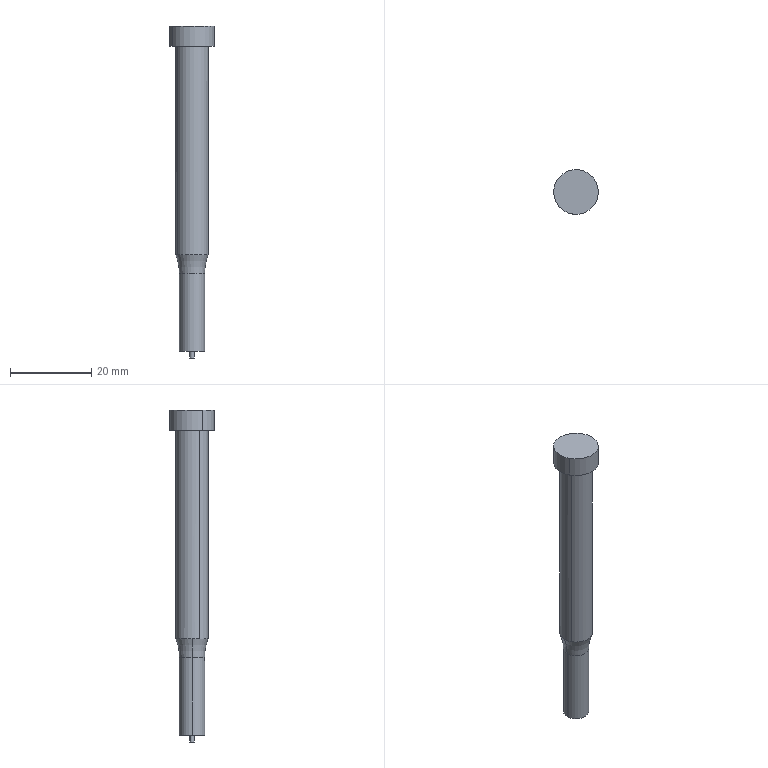Part | CATIA | 1 solid | 14 faces | box 11 x 11 x 81.7 mm | volume 3799 mm3 | cylinder 8 | plane 4 | torus 2 | commonest cylinder face diameters 1.04 x2 6.2 x2 8 x2 11 x2
STEP:
#1=CARTESIAN_POINT('',(3.1,0.,0.));
#2=VERTEX_POINT('',#1);
#3=CARTESIAN_POINT('',(-3.1,0.,0.));
#4=VERTEX_POINT('',#3);
#5=CARTESIAN_POINT('',(0.,0.,0.));
#6=DIRECTION('',(0.,0.,1.));
#7=AXIS2_PLACEMENT_3D('',#5,#6,$);
#8=CIRCLE('',#7,3.1);
#9=EDGE_CURVE('',#2,#4,#8,.T.);
#10=ORIENTED_EDGE('',*,*,#9,.F.);
#11=CARTESIAN_POINT('',(0.,0.,0.));
#12=DIRECTION('',(0.,0.,1.));
#13=AXIS2_PLACEMENT_3D('',#11,#12,$);
#14=CIRCLE('',#13,3.1);
#15=EDGE_CURVE('',#4,#2,#14,.T.);
#16=ORIENTED_EDGE('',*,*,#15,.F.);
#17=EDGE_LOOP('',(#10,#16));
#18=FACE_OUTER_BOUND('',#17,.T.);
#19=CARTESIAN_POINT('',(0.4563,-0.2493,0.));
#20=VERTEX_POINT('',#19);
#21=CARTESIAN_POINT('',(-0.4563,0.2493,0.));
#22=VERTEX_POINT('',#21);
#23=CARTESIAN_POINT('',(0.,0.,0.));
#24=DIRECTION('',(0.,0.,1.));
#25=AXIS2_PLACEMENT_3D('',#23,#24,$);
#26=CIRCLE('',#25,0.52);
#27=EDGE_CURVE('',#20,#22,#26,.F.);
#28=ORIENTED_EDGE('',*,*,#27,.F.);
#29=CARTESIAN_POINT('',(0.,0.,0.));
#30=DIRECTION('',(0.,0.,1.));
#31=AXIS2_PLACEMENT_3D('',#29,#30,$);
#32=CIRCLE('',#31,0.52);
#33=EDGE_CURVE('',#22,#20,#32,.F.);
#34=ORIENTED_EDGE('',*,*,#33,.F.);
#35=EDGE_LOOP('',(#28,#34));
#36=FACE_BOUND('',#35,.T.);
#37=CARTESIAN_POINT('',(4.,0.,0.));
#38=DIRECTION('',(0.,0.,1.));
#39=DIRECTION('',(1.,0.,0.));
#40=AXIS2_PLACEMENT_3D('',#37,#38,#39);
#41=PLANE('',#40);
#42=ADVANCED_FACE('',(#18,#36),#41,.F.);
#43=CARTESIAN_POINT('',(-4.,0.,23.753));
#44=VERTEX_POINT('',#43);
#45=CARTESIAN_POINT('',(3.51,1.918,23.753));
#46=VERTEX_POINT('',#45);
#47=CARTESIAN_POINT('',(0.,0.,23.753));
#48=DIRECTION('',(0.,0.,-1.));
#49=AXIS2_PLACEMENT_3D('',#47,#48,$);
#50=CIRCLE('',#49,4.);
#51=EDGE_CURVE('',#44,#46,#50,.T.);
#52=ORIENTED_EDGE('',*,*,#51,.T.);
#53=CARTESIAN_POINT('',(4.,0.,23.753));
#54=VERTEX_POINT('',#53);
#55=CARTESIAN_POINT('',(0.,0.,23.753));
#56=DIRECTION('',(0.,0.,-1.));
#57=AXIS2_PLACEMENT_3D('',#55,#56,$);
#58=CIRCLE('',#57,4.);
#59=EDGE_CURVE('',#54,#46,#58,.F.);
#60=ORIENTED_EDGE('',*,*,#59,.F.);
#61=CARTESIAN_POINT('',(3.1,0.,19.));
#62=VERTEX_POINT('',#61);
#63=CARTESIAN_POINT('',(16.1,0.,19.));
#64=DIRECTION('',(0.,1.,0.));
#65=AXIS2_PLACEMENT_3D('',#63,#64,$);
#66=CIRCLE('',#65,13.);
#67=EDGE_CURVE('',#54,#62,#66,.F.);
#68=ORIENTED_EDGE('',*,*,#67,.T.);
#69=CARTESIAN_POINT('',(-3.1,0.,19.));
#70=VERTEX_POINT('',#69);
#71=CARTESIAN_POINT('',(0.,0.,19.));
#72=DIRECTION('',(0.,0.,-1.));
#73=AXIS2_PLACEMENT_3D('',#71,#72,$);
#74=CIRCLE('',#73,3.1);
#75=EDGE_CURVE('',#70,#62,#74,.T.);
#76=ORIENTED_EDGE('',*,*,#75,.F.);
#77=CARTESIAN_POINT('',(-16.1,0.,19.));
#78=DIRECTION('',(0.,-1.,0.));
#79=AXIS2_PLACEMENT_3D('',#77,#78,$);
#80=CIRCLE('',#79,13.);
#81=EDGE_CURVE('',#44,#70,#80,.F.);
#82=ORIENTED_EDGE('',*,*,#81,.F.);
#83=EDGE_LOOP('',(#52,#60,#68,#76,#82));
#84=FACE_OUTER_BOUND('',#83,.T.);
#85=CARTESIAN_POINT('',(0.,0.,19.));
#86=DIRECTION('',(0.,0.,-1.));
#87=DIRECTION('',(-0.9862,-0.1654,0.));
#88=AXIS2_PLACEMENT_3D('',#85,#86,#87);
#89=TOROIDAL_SURFACE('',#88,16.1,13.);
#90=ADVANCED_FACE('',(#84),#89,.F.);
#91=CARTESIAN_POINT('',(-3.51,-1.918,23.753));
#92=VERTEX_POINT('',#91);
#93=CARTESIAN_POINT('',(0.,0.,23.753));
#94=DIRECTION('',(0.,0.,-1.));
#95=AXIS2_PLACEMENT_3D('',#93,#94,$);
#96=CIRCLE('',#95,4.);
#97=EDGE_CURVE('',#54,#92,#96,.T.);
#98=ORIENTED_EDGE('',*,*,#97,.T.);
#99=CARTESIAN_POINT('',(0.,0.,23.753));
#100=DIRECTION('',(0.,0.,-1.));
#101=AXIS2_PLACEMENT_3D('',#99,#100,$);
#102=CIRCLE('',#101,4.);
#103=EDGE_CURVE('',#44,#92,#102,.F.);
#104=ORIENTED_EDGE('',*,*,#103,.F.);
#105=ORIENTED_EDGE('',*,*,#81,.T.);
#106=CARTESIAN_POINT('',(0.,0.,19.));
#107=DIRECTION('',(0.,0.,-1.));
#108=AXIS2_PLACEMENT_3D('',#106,#107,$);
#109=CIRCLE('',#108,3.1);
#110=EDGE_CURVE('',#62,#70,#109,.T.);
#111=ORIENTED_EDGE('',*,*,#110,.F.);
#112=ORIENTED_EDGE('',*,*,#67,.F.);
#113=EDGE_LOOP('',(#98,#104,#105,#111,#112));
#114=FACE_OUTER_BOUND('',#113,.T.);
#115=CARTESIAN_POINT('',(0.,0.,19.));
#116=DIRECTION('',(0.,0.,-1.));
#117=DIRECTION('',(0.9734,0.2293,0.));
#118=AXIS2_PLACEMENT_3D('',#115,#116,#117);
#119=TOROIDAL_SURFACE('',#118,16.1,13.);
#120=ADVANCED_FACE('',(#114),#119,.F.);
#121=CARTESIAN_POINT('',(3.1,0.,16.61));
#122=DIRECTION('',(0.,0.,1.));
#123=VECTOR('',#122,1.);
#124=LINE('',#121,#123);
#125=EDGE_CURVE('',#2,#62,#124,.T.);
#126=ORIENTED_EDGE('',*,*,#125,.F.);
#127=ORIENTED_EDGE('',*,*,#9,.T.);
#128=CARTESIAN_POINT('',(-3.1,0.,16.61));
#129=DIRECTION('',(0.,0.,1.));
#130=VECTOR('',#129,1.);
#131=LINE('',#128,#130);
#132=EDGE_CURVE('',#4,#70,#131,.T.);
#133=ORIENTED_EDGE('',*,*,#132,.T.);
#134=ORIENTED_EDGE('',*,*,#75,.T.);
#135=EDGE_LOOP('',(#126,#127,#133,#134));
#136=FACE_OUTER_BOUND('',#135,.T.);
#137=CARTESIAN_POINT('',(0.,0.,16.61));
#138=DIRECTION('',(0.,0.,1.));
#139=DIRECTION('',(1.,0.,0.));
#140=AXIS2_PLACEMENT_3D('',#137,#138,#139);
#141=CYLINDRICAL_SURFACE('',#140,3.1);
#142=ADVANCED_FACE('',(#136),#141,.T.);
#143=ORIENTED_EDGE('',*,*,#132,.F.);
#144=ORIENTED_EDGE('',*,*,#15,.T.);
#145=ORIENTED_EDGE('',*,*,#125,.T.);
#146=ORIENTED_EDGE('',*,*,#110,.T.);
#147=EDGE_LOOP('',(#143,#144,#145,#146));
#148=FACE_OUTER_BOUND('',#147,.T.);
#149=CARTESIAN_POINT('',(0.,0.,16.61));
#150=DIRECTION('',(0.,0.,1.));
#151=DIRECTION('',(-1.,0.,0.));
#152=AXIS2_PLACEMENT_3D('',#149,#150,#151);
#153=CYLINDRICAL_SURFACE('',#152,3.1);
#154=ADVANCED_FACE('',(#148),#153,.T.);
#155=CARTESIAN_POINT('',(-3.51,-1.918,75.));
#156=VERTEX_POINT('',#155);
#157=CARTESIAN_POINT('',(-3.51,-1.918,37.5));
#158=DIRECTION('',(0.,0.,1.));
#159=VECTOR('',#158,1.);
#160=LINE('',#157,#159);
#161=EDGE_CURVE('',#92,#156,#160,.T.);
#162=ORIENTED_EDGE('',*,*,#161,.T.);
#163=CARTESIAN_POINT('',(3.51,1.918,75.));
#164=VERTEX_POINT('',#163);
#165=CARTESIAN_POINT('',(0.,0.,75.));
#166=DIRECTION('',(0.,0.,1.));
#167=AXIS2_PLACEMENT_3D('',#165,#166,$);
#168=CIRCLE('',#167,4.);
#169=EDGE_CURVE('',#164,#156,#168,.T.);
#170=ORIENTED_EDGE('',*,*,#169,.F.);
#171=CARTESIAN_POINT('',(3.51,1.918,37.5));
#172=DIRECTION('',(0.,0.,1.));
#173=VECTOR('',#172,1.);
#174=LINE('',#171,#173);
#175=EDGE_CURVE('',#46,#164,#174,.T.);
#176=ORIENTED_EDGE('',*,*,#175,.F.);
#177=ORIENTED_EDGE('',*,*,#51,.F.);
#178=ORIENTED_EDGE('',*,*,#103,.T.);
#179=EDGE_LOOP('',(#162,#170,#176,#177,#178));
#180=FACE_OUTER_BOUND('',#179,.T.);
#181=CARTESIAN_POINT('',(0.,0.,40.));
#182=DIRECTION('',(0.,0.,1.));
#183=DIRECTION('',(0.8776,0.4794,0.));
#184=AXIS2_PLACEMENT_3D('',#181,#182,#183);
#185=CYLINDRICAL_SURFACE('',#184,4.);
#186=ADVANCED_FACE('',(#180),#185,.T.);
#187=ORIENTED_EDGE('',*,*,#175,.T.);
#188=CARTESIAN_POINT('',(0.,0.,75.));
#189=DIRECTION('',(0.,0.,1.));
#190=AXIS2_PLACEMENT_3D('',#188,#189,$);
#191=CIRCLE('',#190,4.);
#192=EDGE_CURVE('',#156,#164,#191,.T.);
#193=ORIENTED_EDGE('',*,*,#192,.F.);
#194=ORIENTED_EDGE('',*,*,#161,.F.);
#195=ORIENTED_EDGE('',*,*,#97,.F.);
#196=ORIENTED_EDGE('',*,*,#59,.T.);
#197=EDGE_LOOP('',(#187,#193,#194,#195,#196));
#198=FACE_OUTER_BOUND('',#197,.T.);
#199=ADVANCED_FACE('',(#198),#185,.T.);
#200=CARTESIAN_POINT('',(-4.827,-2.637,80.));
#201=VERTEX_POINT('',#200);
#202=CARTESIAN_POINT('',(4.827,2.637,80.));
#203=VERTEX_POINT('',#202);
#204=CARTESIAN_POINT('',(0.,0.,80.));
#205=DIRECTION('',(0.,0.,1.));
#206=AXIS2_PLACEMENT_3D('',#204,#205,$);
#207=CIRCLE('',#206,5.5);
#208=EDGE_CURVE('',#201,#203,#207,.T.);
#209=ORIENTED_EDGE('',*,*,#208,.T.);
#210=CARTESIAN_POINT('',(0.,0.,80.));
#211=DIRECTION('',(0.,0.,1.));
#212=AXIS2_PLACEMENT_3D('',#210,#211,$);
#213=CIRCLE('',#212,5.5);
#214=EDGE_CURVE('',#203,#201,#213,.T.);
#215=ORIENTED_EDGE('',*,*,#214,.T.);
#216=EDGE_LOOP('',(#209,#215));
#217=FACE_OUTER_BOUND('',#216,.T.);
#218=CARTESIAN_POINT('',(0.,0.,80.));
#219=DIRECTION('',(0.,0.,1.));
#220=DIRECTION('',(1.,0.,0.));
#221=AXIS2_PLACEMENT_3D('',#218,#219,#220);
#222=PLANE('',#221);
#223=ADVANCED_FACE('',(#217),#222,.T.);
#224=CARTESIAN_POINT('',(4.827,2.637,75.));
#225=VERTEX_POINT('',#224);
#226=CARTESIAN_POINT('',(-4.827,-2.637,75.));
#227=VERTEX_POINT('',#226);
#228=CARTESIAN_POINT('',(0.,0.,75.));
#229=DIRECTION('',(0.,0.,1.));
#230=AXIS2_PLACEMENT_3D('',#228,#229,$);
#231=CIRCLE('',#230,5.5);
#232=EDGE_CURVE('',#225,#227,#231,.T.);
#233=ORIENTED_EDGE('',*,*,#232,.F.);
#234=CARTESIAN_POINT('',(0.,0.,75.));
#235=DIRECTION('',(0.,0.,1.));
#236=AXIS2_PLACEMENT_3D('',#234,#235,$);
#237=CIRCLE('',#236,5.5);
#238=EDGE_CURVE('',#227,#225,#237,.T.);
#239=ORIENTED_EDGE('',*,*,#238,.F.);
#240=EDGE_LOOP('',(#233,#239));
#241=FACE_OUTER_BOUND('',#240,.T.);
#242=ORIENTED_EDGE('',*,*,#192,.T.);
#243=ORIENTED_EDGE('',*,*,#169,.T.);
#244=EDGE_LOOP('',(#242,#243));
#245=FACE_BOUND('',#244,.T.);
#246=CARTESIAN_POINT('',(5.5,0.,75.));
#247=DIRECTION('',(0.,0.,1.));
#248=DIRECTION('',(1.,0.,0.));
#249=AXIS2_PLACEMENT_3D('',#246,#247,#248);
#250=PLANE('',#249);
#251=ADVANCED_FACE('',(#241,#245),#250,.F.);
#252=CARTESIAN_POINT('',(4.827,2.637,77.5));
#253=DIRECTION('',(0.,0.,1.));
#254=VECTOR('',#253,1.);
#255=LINE('',#252,#254);
#256=EDGE_CURVE('',#225,#203,#255,.T.);
#257=ORIENTED_EDGE('',*,*,#256,.T.);
#258=ORIENTED_EDGE('',*,*,#208,.F.);
#259=CARTESIAN_POINT('',(-4.827,-2.637,77.5));
#260=DIRECTION('',(0.,0.,1.));
#261=VECTOR('',#260,1.);
#262=LINE('',#259,#261);
#263=EDGE_CURVE('',#227,#201,#262,.T.);
#264=ORIENTED_EDGE('',*,*,#263,.F.);
#265=ORIENTED_EDGE('',*,*,#238,.T.);
#266=EDGE_LOOP('',(#257,#258,#264,#265));
#267=FACE_OUTER_BOUND('',#266,.T.);
#268=CARTESIAN_POINT('',(0.,0.,40.));
#269=DIRECTION('',(0.,0.,1.));
#270=DIRECTION('',(0.8776,0.4794,0.));
#271=AXIS2_PLACEMENT_3D('',#268,#269,#270);
#272=CYLINDRICAL_SURFACE('',#271,5.5);
#273=ADVANCED_FACE('',(#267),#272,.T.);
#274=ORIENTED_EDGE('',*,*,#263,.T.);
#275=ORIENTED_EDGE('',*,*,#214,.F.);
#276=ORIENTED_EDGE('',*,*,#256,.F.);
#277=ORIENTED_EDGE('',*,*,#232,.T.);
#278=EDGE_LOOP('',(#274,#275,#276,#277));
#279=FACE_OUTER_BOUND('',#278,.T.);
#280=ADVANCED_FACE('',(#279),#272,.T.);
#281=CARTESIAN_POINT('',(0.4563,-0.2493,-1.7));
#282=VERTEX_POINT('',#281);
#283=CARTESIAN_POINT('',(-0.4563,0.2493,-1.7));
#284=VERTEX_POINT('',#283);
#285=CARTESIAN_POINT('',(0.,0.,-1.7));
#286=DIRECTION('',(0.,0.,-1.));
#287=AXIS2_PLACEMENT_3D('',#285,#286,$);
#288=CIRCLE('',#287,0.52);
#289=EDGE_CURVE('',#282,#284,#288,.T.);
#290=ORIENTED_EDGE('',*,*,#289,.F.);
#291=CARTESIAN_POINT('',(0.4563,-0.2493,-0.85));
#292=DIRECTION('',(0.,0.,-1.));
#293=VECTOR('',#292,1.);
#294=LINE('',#291,#293);
#295=EDGE_CURVE('',#282,#20,#294,.F.);
#296=ORIENTED_EDGE('',*,*,#295,.T.);
#297=ORIENTED_EDGE('',*,*,#27,.T.);
#298=CARTESIAN_POINT('',(-0.4563,0.2493,-0.85));
#299=DIRECTION('',(0.,0.,-1.));
#300=VECTOR('',#299,1.);
#301=LINE('',#298,#300);
#302=EDGE_CURVE('',#284,#22,#301,.F.);
#303=ORIENTED_EDGE('',*,*,#302,.F.);
#304=EDGE_LOOP('',(#290,#296,#297,#303));
#305=FACE_OUTER_BOUND('',#304,.T.);
#306=CARTESIAN_POINT('',(0.,0.,-0.85));
#307=DIRECTION('',(0.,0.,-1.));
#308=DIRECTION('',(0.8776,-0.4794,0.));
#309=AXIS2_PLACEMENT_3D('',#306,#307,#308);
#310=CYLINDRICAL_SURFACE('',#309,0.52);
#311=ADVANCED_FACE('',(#305),#310,.T.);
#312=CARTESIAN_POINT('',(0.,0.,-1.7));
#313=DIRECTION('',(0.,0.,-1.));
#314=AXIS2_PLACEMENT_3D('',#312,#313,$);
#315=CIRCLE('',#314,0.52);
#316=EDGE_CURVE('',#284,#282,#315,.T.);
#317=ORIENTED_EDGE('',*,*,#316,.F.);
#318=ORIENTED_EDGE('',*,*,#302,.T.);
#319=ORIENTED_EDGE('',*,*,#33,.T.);
#320=ORIENTED_EDGE('',*,*,#295,.F.);
#321=EDGE_LOOP('',(#317,#318,#319,#320));
#322=FACE_OUTER_BOUND('',#321,.T.);
#323=ADVANCED_FACE('',(#322),#310,.T.);
#324=ORIENTED_EDGE('',*,*,#289,.T.);
#325=ORIENTED_EDGE('',*,*,#316,.T.);
#326=EDGE_LOOP('',(#324,#325));
#327=FACE_OUTER_BOUND('',#326,.T.);
#328=CARTESIAN_POINT('',(0.52,0.,-1.7));
#329=DIRECTION('',(0.,0.,-1.));
#330=DIRECTION('',(1.,0.,0.));
#331=AXIS2_PLACEMENT_3D('',#328,#329,#330);
#332=PLANE('',#331);
#333=ADVANCED_FACE('',(#327),#332,.T.);
#334=CLOSED_SHELL('',(#42,#90,#120,#142,#154,#186,#199,#223,#251,#273,#280,#311,#323,#333));
#335=MANIFOLD_SOLID_BREP('',#334);
#336=(LENGTH_UNIT()NAMED_UNIT(*)SI_UNIT(.MILLI.,.METRE.));
#337=UNCERTAINTY_MEASURE_WITH_UNIT(LENGTH_MEASURE(0.005),#336,'','');
#338=(NAMED_UNIT(*)PLANE_ANGLE_UNIT()SI_UNIT($,.RADIAN.));
#339=(NAMED_UNIT(*)SI_UNIT($,.STERADIAN.)SOLID_ANGLE_UNIT());
#340=(GEOMETRIC_REPRESENTATION_CONTEXT(3)GLOBAL_UNCERTAINTY_ASSIGNED_CONTEXT((#337))GLOBAL_UNIT_ASSIGNED_CONTEXT((#336,#338,#339))REPRESENTATION_CONTEXT('',''));
#341=ADVANCED_BREP_SHAPE_REPRESENTATION('',(#335),#340);